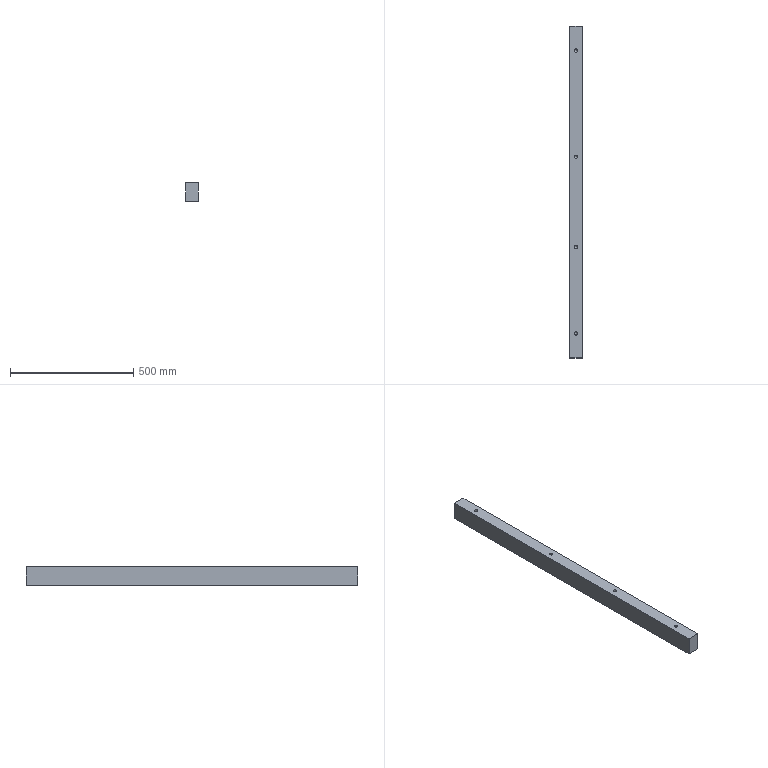Part | NX | features 3 2 | 1 solid | 22 faces | box 50 x 1345 x 75.5 mm | volume 5064509 mm3 | cylinder 8 | cone 8 | plane 6 | commonest cylinder face diameters 14.1 x8
STEP:
#1=CARTESIAN_POINT('',(537.05,572.5,256.5));
#2=VERTEX_POINT('',#1);
#3=CARTESIAN_POINT('',(530.,572.5,256.5));
#4=DIRECTION('',(0.,0.,-1.));
#5=DIRECTION('',(1.,0.,0.));
#6=AXIS2_PLACEMENT_3D('',#3,#4,#5);
#7=CIRCLE('',#6,7.05);
#8=EDGE_CURVE('',#2,#2,#7,.T.);
#9=ORIENTED_EDGE('',*,*,#8,.T.);
#10=EDGE_LOOP('',(#9));
#11=FACE_BOUND('',#10,.T.);
#12=CARTESIAN_POINT('',(537.05,-572.5,256.5));
#13=VERTEX_POINT('',#12);
#14=CARTESIAN_POINT('',(530.,-572.5,256.5));
#15=DIRECTION('',(0.,0.,-1.));
#16=DIRECTION('',(1.,0.,0.));
#17=AXIS2_PLACEMENT_3D('',#14,#15,#16);
#18=CIRCLE('',#17,7.05);
#19=EDGE_CURVE('',#13,#13,#18,.T.);
#20=ORIENTED_EDGE('',*,*,#19,.T.);
#21=EDGE_LOOP('',(#20));
#22=FACE_BOUND('',#21,.T.);
#23=CARTESIAN_POINT('',(555.,-672.5,256.5));
#24=VERTEX_POINT('',#23);
#25=CARTESIAN_POINT('',(505.,-672.5,256.5));
#26=VERTEX_POINT('',#25);
#27=CARTESIAN_POINT('',(282.5,-672.5,256.5));
#28=DIRECTION('',(-1.,0.,0.));
#29=VECTOR('',#28,1000.);
#30=LINE('',#27,#29);
#31=EDGE_CURVE('',#24,#26,#30,.T.);
#32=ORIENTED_EDGE('',*,*,#31,.F.);
#33=CARTESIAN_POINT('',(555.,672.5,256.5));
#34=VERTEX_POINT('',#33);
#35=CARTESIAN_POINT('',(555.,193.,256.5));
#36=DIRECTION('',(0.,-1.,0.));
#37=VECTOR('',#36,1000.);
#38=LINE('',#35,#37);
#39=EDGE_CURVE('',#34,#24,#38,.T.);
#40=ORIENTED_EDGE('',*,*,#39,.F.);
#41=CARTESIAN_POINT('',(505.,672.5,256.5));
#42=VERTEX_POINT('',#41);
#43=CARTESIAN_POINT('',(505.,672.5,256.5));
#44=DIRECTION('',(1.,0.,0.));
#45=VECTOR('',#44,1000.);
#46=LINE('',#43,#45);
#47=EDGE_CURVE('',#42,#34,#46,.T.);
#48=ORIENTED_EDGE('',*,*,#47,.F.);
#49=CARTESIAN_POINT('',(505.,193.,256.5));
#50=DIRECTION('',(0.,1.,0.));
#51=VECTOR('',#50,1000.);
#52=LINE('',#49,#51);
#53=EDGE_CURVE('',#26,#42,#52,.T.);
#54=ORIENTED_EDGE('',*,*,#53,.F.);
#55=EDGE_LOOP('',(#32,#40,#48,#54));
#56=FACE_BOUND('',#55,.T.);
#57=CARTESIAN_POINT('',(537.05,-222.5,256.5));
#58=VERTEX_POINT('',#57);
#59=CARTESIAN_POINT('',(530.,-222.5,256.5));
#60=DIRECTION('',(0.,0.,-1.));
#61=DIRECTION('',(1.,0.,0.));
#62=AXIS2_PLACEMENT_3D('',#59,#60,#61);
#63=CIRCLE('',#62,7.05);
#64=EDGE_CURVE('',#58,#58,#63,.T.);
#65=ORIENTED_EDGE('',*,*,#64,.T.);
#66=EDGE_LOOP('',(#65));
#67=FACE_BOUND('',#66,.T.);
#68=CARTESIAN_POINT('',(537.05,142.5,256.5));
#69=VERTEX_POINT('',#68);
#70=CARTESIAN_POINT('',(530.,142.5,256.5));
#71=DIRECTION('',(0.,0.,-1.));
#72=DIRECTION('',(1.,0.,0.));
#73=AXIS2_PLACEMENT_3D('',#70,#71,#72);
#74=CIRCLE('',#73,7.05);
#75=EDGE_CURVE('',#69,#69,#74,.T.);
#76=ORIENTED_EDGE('',*,*,#75,.T.);
#77=EDGE_LOOP('',(#76));
#78=FACE_BOUND('',#77,.T.);
#79=CARTESIAN_POINT('',(2545.,0.,256.5));
#80=DIRECTION('',(0.,0.,1.));
#81=DIRECTION('',(-1.,0.,0.));
#82=AXIS2_PLACEMENT_3D('',#79,#80,#81);
#83=PLANE('',#82);
#84=ADVANCED_FACE('',(#11,#22,#56,#67,#78),#83,.T.);
#85=CARTESIAN_POINT('',(537.05,142.5,181.));
#86=VERTEX_POINT('',#85);
#87=CARTESIAN_POINT('',(530.,142.5,181.));
#88=DIRECTION('',(0.,0.,1.));
#89=DIRECTION('',(1.,0.,0.));
#90=AXIS2_PLACEMENT_3D('',#87,#88,#89);
#91=CIRCLE('',#90,7.05);
#92=EDGE_CURVE('',#86,#86,#91,.T.);
#93=ORIENTED_EDGE('',*,*,#92,.T.);
#94=EDGE_LOOP('',(#93));
#95=FACE_BOUND('',#94,.T.);
#96=CARTESIAN_POINT('',(537.05,-222.5,181.));
#97=VERTEX_POINT('',#96);
#98=CARTESIAN_POINT('',(530.,-222.5,181.));
#99=DIRECTION('',(0.,0.,1.));
#100=DIRECTION('',(1.,0.,0.));
#101=AXIS2_PLACEMENT_3D('',#98,#99,#100);
#102=CIRCLE('',#101,7.05);
#103=EDGE_CURVE('',#97,#97,#102,.T.);
#104=ORIENTED_EDGE('',*,*,#103,.T.);
#105=EDGE_LOOP('',(#104));
#106=FACE_BOUND('',#105,.T.);
#107=CARTESIAN_POINT('',(505.,672.5,181.));
#108=VERTEX_POINT('',#107);
#109=CARTESIAN_POINT('',(505.,-672.5,181.));
#110=VERTEX_POINT('',#109);
#111=CARTESIAN_POINT('',(505.,193.,181.));
#112=DIRECTION('',(0.,-1.,0.));
#113=VECTOR('',#112,1000.);
#114=LINE('',#111,#113);
#115=EDGE_CURVE('',#108,#110,#114,.T.);
#116=ORIENTED_EDGE('',*,*,#115,.F.);
#117=CARTESIAN_POINT('',(555.,672.5,181.));
#118=VERTEX_POINT('',#117);
#119=CARTESIAN_POINT('',(1775.,672.5,181.));
#120=DIRECTION('',(1.,0.,0.));
#121=VECTOR('',#120,1000.);
#122=LINE('',#119,#121);
#123=EDGE_CURVE('',#108,#118,#122,.T.);
#124=ORIENTED_EDGE('',*,*,#123,.T.);
#125=CARTESIAN_POINT('',(555.,-672.5,181.));
#126=VERTEX_POINT('',#125);
#127=CARTESIAN_POINT('',(555.,193.,181.));
#128=DIRECTION('',(0.,1.,0.));
#129=VECTOR('',#128,1000.);
#130=LINE('',#127,#129);
#131=EDGE_CURVE('',#126,#118,#130,.T.);
#132=ORIENTED_EDGE('',*,*,#131,.F.);
#133=CARTESIAN_POINT('',(1775.,-672.5,181.));
#134=DIRECTION('',(-1.,0.,0.));
#135=VECTOR('',#134,1000.);
#136=LINE('',#133,#135);
#137=EDGE_CURVE('',#126,#110,#136,.T.);
#138=ORIENTED_EDGE('',*,*,#137,.T.);
#139=EDGE_LOOP('',(#116,#124,#132,#138));
#140=FACE_BOUND('',#139,.T.);
#141=CARTESIAN_POINT('',(537.05,-572.5,181.));
#142=VERTEX_POINT('',#141);
#143=CARTESIAN_POINT('',(530.,-572.5,181.));
#144=DIRECTION('',(0.,0.,1.));
#145=DIRECTION('',(1.,0.,0.));
#146=AXIS2_PLACEMENT_3D('',#143,#144,#145);
#147=CIRCLE('',#146,7.05);
#148=EDGE_CURVE('',#142,#142,#147,.T.);
#149=ORIENTED_EDGE('',*,*,#148,.T.);
#150=EDGE_LOOP('',(#149));
#151=FACE_BOUND('',#150,.T.);
#152=CARTESIAN_POINT('',(537.05,572.5,181.));
#153=VERTEX_POINT('',#152);
#154=CARTESIAN_POINT('',(530.,572.5,181.));
#155=DIRECTION('',(0.,0.,1.));
#156=DIRECTION('',(1.,0.,0.));
#157=AXIS2_PLACEMENT_3D('',#154,#155,#156);
#158=CIRCLE('',#157,7.05);
#159=EDGE_CURVE('',#153,#153,#158,.T.);
#160=ORIENTED_EDGE('',*,*,#159,.T.);
#161=EDGE_LOOP('',(#160));
#162=FACE_BOUND('',#161,.T.);
#163=CARTESIAN_POINT('',(1775.,193.,181.));
#164=DIRECTION('',(0.,0.,-1.));
#165=DIRECTION('',(-1.,0.,0.));
#166=AXIS2_PLACEMENT_3D('',#163,#164,#165);
#167=PLANE('',#166);
#168=ADVANCED_FACE('',(#95,#106,#140,#151,#162),#167,.T.);
#169=CARTESIAN_POINT('',(505.,-672.5,-1.5));
#170=DIRECTION('',(0.,0.,1.));
#171=VECTOR('',#170,1000.);
#172=LINE('',#169,#171);
#173=EDGE_CURVE('',#110,#26,#172,.T.);
#174=ORIENTED_EDGE('',*,*,#173,.T.);
#175=ORIENTED_EDGE('',*,*,#53,.T.);
#176=CARTESIAN_POINT('',(505.,672.5,-1.5));
#177=DIRECTION('',(0.,0.,-1.));
#178=VECTOR('',#177,1000.);
#179=LINE('',#176,#178);
#180=EDGE_CURVE('',#42,#108,#179,.T.);
#181=ORIENTED_EDGE('',*,*,#180,.T.);
#182=ORIENTED_EDGE('',*,*,#115,.T.);
#183=EDGE_LOOP('',(#174,#175,#181,#182));
#184=FACE_BOUND('',#183,.T.);
#185=CARTESIAN_POINT('',(505.,193.,-1.5));
#186=DIRECTION('',(-1.,0.,0.));
#187=DIRECTION('',(0.,0.,-1.));
#188=AXIS2_PLACEMENT_3D('',#185,#186,#187);
#189=PLANE('',#188);
#190=ADVANCED_FACE('',(#184),#189,.T.);
#191=CARTESIAN_POINT('',(555.,672.5,-1.5));
#192=DIRECTION('',(0.,0.,1.));
#193=VECTOR('',#192,1000.);
#194=LINE('',#191,#193);
#195=EDGE_CURVE('',#118,#34,#194,.T.);
#196=ORIENTED_EDGE('',*,*,#195,.T.);
#197=ORIENTED_EDGE('',*,*,#39,.T.);
#198=CARTESIAN_POINT('',(555.,-672.5,-1.5));
#199=DIRECTION('',(0.,0.,-1.));
#200=VECTOR('',#199,1000.);
#201=LINE('',#198,#200);
#202=EDGE_CURVE('',#24,#126,#201,.T.);
#203=ORIENTED_EDGE('',*,*,#202,.T.);
#204=ORIENTED_EDGE('',*,*,#131,.T.);
#205=EDGE_LOOP('',(#196,#197,#203,#204));
#206=FACE_BOUND('',#205,.T.);
#207=CARTESIAN_POINT('',(555.,193.,-1.5));
#208=DIRECTION('',(1.,0.,0.));
#209=DIRECTION('',(0.,0.,1.));
#210=AXIS2_PLACEMENT_3D('',#207,#208,#209);
#211=PLANE('',#210);
#212=ADVANCED_FACE('',(#206),#211,.T.);
#213=ORIENTED_EDGE('',*,*,#202,.F.);
#214=ORIENTED_EDGE('',*,*,#31,.T.);
#215=ORIENTED_EDGE('',*,*,#173,.F.);
#216=ORIENTED_EDGE('',*,*,#137,.F.);
#217=EDGE_LOOP('',(#213,#214,#215,#216));
#218=FACE_BOUND('',#217,.T.);
#219=CARTESIAN_POINT('',(282.5,-672.5,-103.));
#220=DIRECTION('',(0.,1.,0.));
#221=DIRECTION('',(1.,0.,0.));
#222=AXIS2_PLACEMENT_3D('',#219,#220,#221);
#223=PLANE('',#222);
#224=ADVANCED_FACE('',(#218),#223,.F.);
#225=ORIENTED_EDGE('',*,*,#180,.F.);
#226=ORIENTED_EDGE('',*,*,#47,.T.);
#227=ORIENTED_EDGE('',*,*,#195,.F.);
#228=ORIENTED_EDGE('',*,*,#123,.F.);
#229=EDGE_LOOP('',(#225,#226,#227,#228));
#230=FACE_BOUND('',#229,.T.);
#231=CARTESIAN_POINT('',(505.,672.5,231.5));
#232=DIRECTION('',(0.,1.,0.));
#233=DIRECTION('',(0.,0.,-1.));
#234=AXIS2_PLACEMENT_3D('',#231,#232,#233);
#235=PLANE('',#234);
#236=ADVANCED_FACE('',(#230),#235,.T.);
#237=ORIENTED_EDGE('',*,*,#103,.F.);
#238=EDGE_LOOP('',(#237));
#239=FACE_BOUND('',#238,.T.);
#240=CARTESIAN_POINT('',(537.05,-222.5,188.95));
#241=VERTEX_POINT('',#240);
#242=CARTESIAN_POINT('',(530.,-222.5,188.95));
#243=DIRECTION('',(0.,0.,-1.));
#244=DIRECTION('',(1.,0.,0.));
#245=AXIS2_PLACEMENT_3D('',#242,#243,#244);
#246=CIRCLE('',#245,7.05);
#247=EDGE_CURVE('',#241,#241,#246,.T.);
#248=ORIENTED_EDGE('',*,*,#247,.F.);
#249=EDGE_LOOP('',(#248));
#250=FACE_BOUND('',#249,.T.);
#251=CARTESIAN_POINT('',(530.,-222.5,181.));
#252=DIRECTION('',(0.,0.,1.));
#253=DIRECTION('',(-1.,0.,0.));
#254=AXIS2_PLACEMENT_3D('',#251,#252,#253);
#255=CYLINDRICAL_SURFACE('',#254,7.05);
#256=ADVANCED_FACE('',(#239,#250),#255,.F.);
#257=ORIENTED_EDGE('',*,*,#148,.F.);
#258=EDGE_LOOP('',(#257));
#259=FACE_BOUND('',#258,.T.);
#260=CARTESIAN_POINT('',(537.05,-572.5,188.95));
#261=VERTEX_POINT('',#260);
#262=CARTESIAN_POINT('',(530.,-572.5,188.95));
#263=DIRECTION('',(0.,0.,-1.));
#264=DIRECTION('',(1.,0.,0.));
#265=AXIS2_PLACEMENT_3D('',#262,#263,#264);
#266=CIRCLE('',#265,7.05);
#267=EDGE_CURVE('',#261,#261,#266,.T.);
#268=ORIENTED_EDGE('',*,*,#267,.F.);
#269=EDGE_LOOP('',(#268));
#270=FACE_BOUND('',#269,.T.);
#271=CARTESIAN_POINT('',(530.,-572.5,181.));
#272=DIRECTION('',(0.,0.,1.));
#273=DIRECTION('',(-1.,0.,0.));
#274=AXIS2_PLACEMENT_3D('',#271,#272,#273);
#275=CYLINDRICAL_SURFACE('',#274,7.05);
#276=ADVANCED_FACE('',(#259,#270),#275,.F.);
#277=ORIENTED_EDGE('',*,*,#92,.F.);
#278=EDGE_LOOP('',(#277));
#279=FACE_BOUND('',#278,.T.);
#280=CARTESIAN_POINT('',(537.05,142.5,188.95));
#281=VERTEX_POINT('',#280);
#282=CARTESIAN_POINT('',(530.,142.5,188.95));
#283=DIRECTION('',(0.,0.,-1.));
#284=DIRECTION('',(1.,0.,0.));
#285=AXIS2_PLACEMENT_3D('',#282,#283,#284);
#286=CIRCLE('',#285,7.05);
#287=EDGE_CURVE('',#281,#281,#286,.T.);
#288=ORIENTED_EDGE('',*,*,#287,.F.);
#289=EDGE_LOOP('',(#288));
#290=FACE_BOUND('',#289,.T.);
#291=CARTESIAN_POINT('',(530.,142.5,181.));
#292=DIRECTION('',(0.,0.,1.));
#293=DIRECTION('',(-1.,0.,0.));
#294=AXIS2_PLACEMENT_3D('',#291,#292,#293);
#295=CYLINDRICAL_SURFACE('',#294,7.05);
#296=ADVANCED_FACE('',(#279,#290),#295,.F.);
#297=ORIENTED_EDGE('',*,*,#159,.F.);
#298=EDGE_LOOP('',(#297));
#299=FACE_BOUND('',#298,.T.);
#300=CARTESIAN_POINT('',(537.05,572.5,188.95));
#301=VERTEX_POINT('',#300);
#302=CARTESIAN_POINT('',(530.,572.5,188.95));
#303=DIRECTION('',(0.,0.,-1.));
#304=DIRECTION('',(1.,0.,0.));
#305=AXIS2_PLACEMENT_3D('',#302,#303,#304);
#306=CIRCLE('',#305,7.05);
#307=EDGE_CURVE('',#301,#301,#306,.T.);
#308=ORIENTED_EDGE('',*,*,#307,.F.);
#309=EDGE_LOOP('',(#308));
#310=FACE_BOUND('',#309,.T.);
#311=CARTESIAN_POINT('',(530.,572.5,181.));
#312=DIRECTION('',(0.,0.,1.));
#313=DIRECTION('',(-1.,0.,0.));
#314=AXIS2_PLACEMENT_3D('',#311,#312,#313);
#315=CYLINDRICAL_SURFACE('',#314,7.05);
#316=ADVANCED_FACE('',(#299,#310),#315,.F.);
#317=CARTESIAN_POINT('',(530.,-222.5,196.));
#318=VERTEX_POINT('',#317);
#319=VERTEX_LOOP('',#318);
#320=FACE_BOUND('',#319,.T.);
#321=ORIENTED_EDGE('',*,*,#247,.T.);
#322=EDGE_LOOP('',(#321));
#323=FACE_BOUND('',#322,.T.);
#324=CARTESIAN_POINT('',(530.,-222.5,188.95));
#325=DIRECTION('',(0.,0.,-1.));
#326=DIRECTION('',(1.,0.,0.));
#327=AXIS2_PLACEMENT_3D('',#324,#325,#326);
#328=CONICAL_SURFACE('',#327,7.05,0.7854);
#329=ADVANCED_FACE('',(#320,#323),#328,.F.);
#330=CARTESIAN_POINT('',(530.,-572.5,196.));
#331=VERTEX_POINT('',#330);
#332=VERTEX_LOOP('',#331);
#333=FACE_BOUND('',#332,.T.);
#334=ORIENTED_EDGE('',*,*,#267,.T.);
#335=EDGE_LOOP('',(#334));
#336=FACE_BOUND('',#335,.T.);
#337=CARTESIAN_POINT('',(530.,-572.5,188.95));
#338=DIRECTION('',(0.,0.,-1.));
#339=DIRECTION('',(1.,0.,0.));
#340=AXIS2_PLACEMENT_3D('',#337,#338,#339);
#341=CONICAL_SURFACE('',#340,7.05,0.7854);
#342=ADVANCED_FACE('',(#333,#336),#341,.F.);
#343=CARTESIAN_POINT('',(530.,142.5,196.));
#344=VERTEX_POINT('',#343);
#345=VERTEX_LOOP('',#344);
#346=FACE_BOUND('',#345,.T.);
#347=ORIENTED_EDGE('',*,*,#287,.T.);
#348=EDGE_LOOP('',(#347));
#349=FACE_BOUND('',#348,.T.);
#350=CARTESIAN_POINT('',(530.,142.5,188.95));
#351=DIRECTION('',(0.,0.,-1.));
#352=DIRECTION('',(1.,0.,0.));
#353=AXIS2_PLACEMENT_3D('',#350,#351,#352);
#354=CONICAL_SURFACE('',#353,7.05,0.7854);
#355=ADVANCED_FACE('',(#346,#349),#354,.F.);
#356=CARTESIAN_POINT('',(530.,572.5,196.));
#357=VERTEX_POINT('',#356);
#358=VERTEX_LOOP('',#357);
#359=FACE_BOUND('',#358,.T.);
#360=ORIENTED_EDGE('',*,*,#307,.T.);
#361=EDGE_LOOP('',(#360));
#362=FACE_BOUND('',#361,.T.);
#363=CARTESIAN_POINT('',(530.,572.5,188.95));
#364=DIRECTION('',(0.,0.,-1.));
#365=DIRECTION('',(1.,0.,0.));
#366=AXIS2_PLACEMENT_3D('',#363,#364,#365);
#367=CONICAL_SURFACE('',#366,7.05,0.7854);
#368=ADVANCED_FACE('',(#359,#362),#367,.F.);
#369=CARTESIAN_POINT('',(522.95,-572.5,248.55));
#370=VERTEX_POINT('',#369);
#371=CARTESIAN_POINT('',(530.,-572.5,248.55));
#372=DIRECTION('',(0.,0.,-1.));
#373=DIRECTION('',(-1.,0.,0.));
#374=AXIS2_PLACEMENT_3D('',#371,#372,#373);
#375=CIRCLE('',#374,7.05);
#376=EDGE_CURVE('',#370,#370,#375,.T.);
#377=ORIENTED_EDGE('',*,*,#376,.T.);
#378=EDGE_LOOP('',(#377));
#379=FACE_BOUND('',#378,.T.);
#380=ORIENTED_EDGE('',*,*,#19,.F.);
#381=EDGE_LOOP('',(#380));
#382=FACE_BOUND('',#381,.T.);
#383=CARTESIAN_POINT('',(530.,-572.5,256.5));
#384=DIRECTION('',(0.,0.,-1.));
#385=DIRECTION('',(-1.,0.,0.));
#386=AXIS2_PLACEMENT_3D('',#383,#384,#385);
#387=CYLINDRICAL_SURFACE('',#386,7.05);
#388=ADVANCED_FACE('',(#379,#382),#387,.F.);
#389=CARTESIAN_POINT('',(530.,-572.5,241.5));
#390=VERTEX_POINT('',#389);
#391=VERTEX_LOOP('',#390);
#392=FACE_BOUND('',#391,.T.);
#393=ORIENTED_EDGE('',*,*,#376,.F.);
#394=EDGE_LOOP('',(#393));
#395=FACE_BOUND('',#394,.T.);
#396=CARTESIAN_POINT('',(530.,-572.5,248.55));
#397=DIRECTION('',(0.,0.,1.));
#398=DIRECTION('',(-1.,0.,0.));
#399=AXIS2_PLACEMENT_3D('',#396,#397,#398);
#400=CONICAL_SURFACE('',#399,7.05,0.7854);
#401=ADVANCED_FACE('',(#392,#395),#400,.F.);
#402=CARTESIAN_POINT('',(522.95,-222.5,248.55));
#403=VERTEX_POINT('',#402);
#404=CARTESIAN_POINT('',(530.,-222.5,248.55));
#405=DIRECTION('',(0.,0.,-1.));
#406=DIRECTION('',(-1.,0.,0.));
#407=AXIS2_PLACEMENT_3D('',#404,#405,#406);
#408=CIRCLE('',#407,7.05);
#409=EDGE_CURVE('',#403,#403,#408,.T.);
#410=ORIENTED_EDGE('',*,*,#409,.T.);
#411=EDGE_LOOP('',(#410));
#412=FACE_BOUND('',#411,.T.);
#413=ORIENTED_EDGE('',*,*,#64,.F.);
#414=EDGE_LOOP('',(#413));
#415=FACE_BOUND('',#414,.T.);
#416=CARTESIAN_POINT('',(530.,-222.5,256.5));
#417=DIRECTION('',(0.,0.,-1.));
#418=DIRECTION('',(-1.,0.,0.));
#419=AXIS2_PLACEMENT_3D('',#416,#417,#418);
#420=CYLINDRICAL_SURFACE('',#419,7.05);
#421=ADVANCED_FACE('',(#412,#415),#420,.F.);
#422=CARTESIAN_POINT('',(530.,-222.5,241.5));
#423=VERTEX_POINT('',#422);
#424=VERTEX_LOOP('',#423);
#425=FACE_BOUND('',#424,.T.);
#426=ORIENTED_EDGE('',*,*,#409,.F.);
#427=EDGE_LOOP('',(#426));
#428=FACE_BOUND('',#427,.T.);
#429=CARTESIAN_POINT('',(530.,-222.5,248.55));
#430=DIRECTION('',(0.,0.,1.));
#431=DIRECTION('',(-1.,0.,0.));
#432=AXIS2_PLACEMENT_3D('',#429,#430,#431);
#433=CONICAL_SURFACE('',#432,7.05,0.7854);
#434=ADVANCED_FACE('',(#425,#428),#433,.F.);
#435=CARTESIAN_POINT('',(522.95,572.5,248.55));
#436=VERTEX_POINT('',#435);
#437=CARTESIAN_POINT('',(530.,572.5,248.55));
#438=DIRECTION('',(0.,0.,-1.));
#439=DIRECTION('',(-1.,0.,0.));
#440=AXIS2_PLACEMENT_3D('',#437,#438,#439);
#441=CIRCLE('',#440,7.05);
#442=EDGE_CURVE('',#436,#436,#441,.T.);
#443=ORIENTED_EDGE('',*,*,#442,.T.);
#444=EDGE_LOOP('',(#443));
#445=FACE_BOUND('',#444,.T.);
#446=ORIENTED_EDGE('',*,*,#8,.F.);
#447=EDGE_LOOP('',(#446));
#448=FACE_BOUND('',#447,.T.);
#449=CARTESIAN_POINT('',(530.,572.5,256.5));
#450=DIRECTION('',(0.,0.,-1.));
#451=DIRECTION('',(-1.,0.,0.));
#452=AXIS2_PLACEMENT_3D('',#449,#450,#451);
#453=CYLINDRICAL_SURFACE('',#452,7.05);
#454=ADVANCED_FACE('',(#445,#448),#453,.F.);
#455=CARTESIAN_POINT('',(530.,572.5,241.5));
#456=VERTEX_POINT('',#455);
#457=VERTEX_LOOP('',#456);
#458=FACE_BOUND('',#457,.T.);
#459=ORIENTED_EDGE('',*,*,#442,.F.);
#460=EDGE_LOOP('',(#459));
#461=FACE_BOUND('',#460,.T.);
#462=CARTESIAN_POINT('',(530.,572.5,248.55));
#463=DIRECTION('',(0.,0.,1.));
#464=DIRECTION('',(-1.,0.,0.));
#465=AXIS2_PLACEMENT_3D('',#462,#463,#464);
#466=CONICAL_SURFACE('',#465,7.05,0.7854);
#467=ADVANCED_FACE('',(#458,#461),#466,.F.);
#468=CARTESIAN_POINT('',(522.95,142.5,248.55));
#469=VERTEX_POINT('',#468);
#470=CARTESIAN_POINT('',(530.,142.5,248.55));
#471=DIRECTION('',(0.,0.,-1.));
#472=DIRECTION('',(-1.,0.,0.));
#473=AXIS2_PLACEMENT_3D('',#470,#471,#472);
#474=CIRCLE('',#473,7.05);
#475=EDGE_CURVE('',#469,#469,#474,.T.);
#476=ORIENTED_EDGE('',*,*,#475,.T.);
#477=EDGE_LOOP('',(#476));
#478=FACE_BOUND('',#477,.T.);
#479=ORIENTED_EDGE('',*,*,#75,.F.);
#480=EDGE_LOOP('',(#479));
#481=FACE_BOUND('',#480,.T.);
#482=CARTESIAN_POINT('',(530.,142.5,256.5));
#483=DIRECTION('',(0.,0.,-1.));
#484=DIRECTION('',(-1.,0.,0.));
#485=AXIS2_PLACEMENT_3D('',#482,#483,#484);
#486=CYLINDRICAL_SURFACE('',#485,7.05);
#487=ADVANCED_FACE('',(#478,#481),#486,.F.);
#488=CARTESIAN_POINT('',(530.,142.5,241.5));
#489=VERTEX_POINT('',#488);
#490=VERTEX_LOOP('',#489);
#491=FACE_BOUND('',#490,.T.);
#492=ORIENTED_EDGE('',*,*,#475,.F.);
#493=EDGE_LOOP('',(#492));
#494=FACE_BOUND('',#493,.T.);
#495=CARTESIAN_POINT('',(530.,142.5,248.55));
#496=DIRECTION('',(0.,0.,1.));
#497=DIRECTION('',(-1.,0.,0.));
#498=AXIS2_PLACEMENT_3D('',#495,#496,#497);
#499=CONICAL_SURFACE('',#498,7.05,0.7854);
#500=ADVANCED_FACE('',(#491,#494),#499,.F.);
#501=CLOSED_SHELL('',(#84,#168,#190,#212,#224,#236,#256,#276,#296,#316,#329,#342,#355,#368,#388,#401,#421,#434,#454,#467,#487,#500));
#502=MANIFOLD_SOLID_BREP('',#501);
#503=(LENGTH_UNIT()NAMED_UNIT(*)SI_UNIT(.MILLI.,.METRE.));
#504=UNCERTAINTY_MEASURE_WITH_UNIT(LENGTH_MEASURE(0.00001),#503,'','');
#505=(NAMED_UNIT(*)PLANE_ANGLE_UNIT()SI_UNIT($,.RADIAN.));
#506=(NAMED_UNIT(*)SI_UNIT($,.STERADIAN.)SOLID_ANGLE_UNIT());
#507=(GEOMETRIC_REPRESENTATION_CONTEXT(3)GLOBAL_UNCERTAINTY_ASSIGNED_CONTEXT((#504))GLOBAL_UNIT_ASSIGNED_CONTEXT((#503,#505,#506))REPRESENTATION_CONTEXT('',''));
#508=ADVANCED_BREP_SHAPE_REPRESENTATION('',(#502),#507);